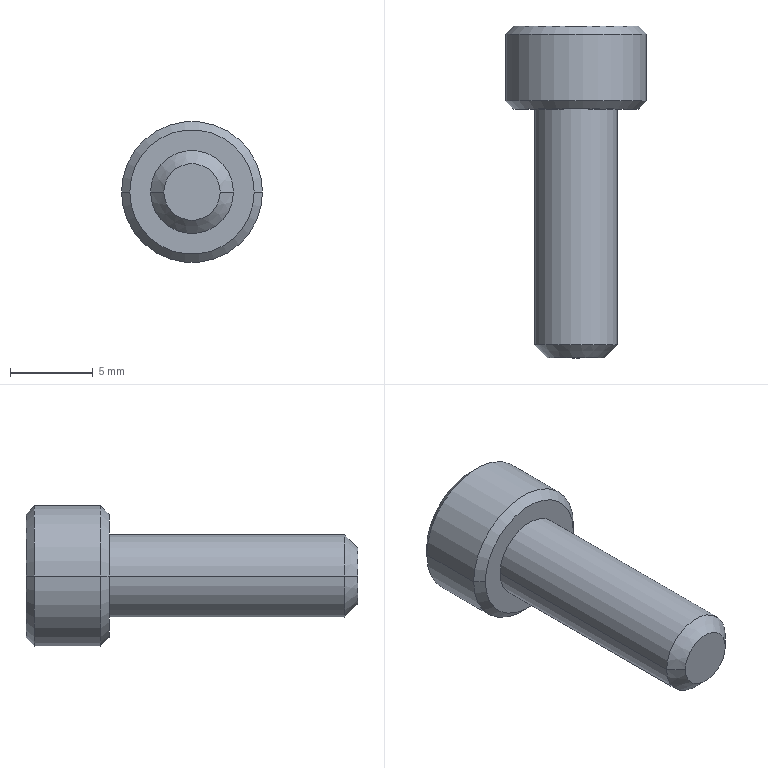Part | STEP file | BB62-M5-15L-1 | 1 solid | 27 faces | box 8.5 x 20 x 8.5 mm | volume 526.023 mm3 | plane 15 | cone 8 | cylinder 4 | commonest cylinder face diameters 5 x2 8.5 x2
STEP:
#1=CARTESIAN_POINT('',(0.,1.178,0.));
#2=VERTEX_POINT('',#1);
#3=CARTESIAN_POINT('',(2.29,2.5,0.));
#4=VERTEX_POINT('',#3);
#5=CARTESIAN_POINT('',(0.,1.178,0.));
#6=DIRECTION('',(0.866,0.5,0.));
#7=VECTOR('',#6,1000.);
#8=LINE('',#5,#7);
#9=EDGE_CURVE('',#2,#4,#8,.T.);
#10=ORIENTED_EDGE('',*,*,#9,.F.);
#11=CARTESIAN_POINT('',(-2.29,2.5,0.));
#12=VERTEX_POINT('',#11);
#13=CARTESIAN_POINT('',(0.,1.178,0.));
#14=DIRECTION('',(-0.866,0.5,0.));
#15=VECTOR('',#14,1000.);
#16=LINE('',#13,#15);
#17=EDGE_CURVE('',#2,#12,#16,.T.);
#18=ORIENTED_EDGE('',*,*,#17,.T.);
#19=CARTESIAN_POINT('',(-1.983,2.5,1.145));
#20=VERTEX_POINT('',#19);
#21=CARTESIAN_POINT('',(0.,2.5,0.));
#22=DIRECTION('',(0.,-1.,0.));
#23=DIRECTION('',(-1.,0.,0.));
#24=AXIS2_PLACEMENT_3D('',#21,#22,#23);
#25=CIRCLE('',#24,2.29);
#26=EDGE_CURVE('',#20,#12,#25,.T.);
#27=ORIENTED_EDGE('',*,*,#26,.F.);
#28=CARTESIAN_POINT('',(0.,2.5,2.29));
#29=VERTEX_POINT('',#28);
#30=CARTESIAN_POINT('',(0.,2.5,0.));
#31=DIRECTION('',(0.,-1.,0.));
#32=DIRECTION('',(-1.,0.,0.));
#33=AXIS2_PLACEMENT_3D('',#30,#31,#32);
#34=CIRCLE('',#33,2.29);
#35=EDGE_CURVE('',#29,#20,#34,.T.);
#36=ORIENTED_EDGE('',*,*,#35,.F.);
#37=CARTESIAN_POINT('',(1.983,2.5,1.145));
#38=VERTEX_POINT('',#37);
#39=CARTESIAN_POINT('',(0.,2.5,0.));
#40=DIRECTION('',(0.,-1.,0.));
#41=DIRECTION('',(-1.,0.,0.));
#42=AXIS2_PLACEMENT_3D('',#39,#40,#41);
#43=CIRCLE('',#42,2.29);
#44=EDGE_CURVE('',#38,#29,#43,.T.);
#45=ORIENTED_EDGE('',*,*,#44,.F.);
#46=CARTESIAN_POINT('',(0.,2.5,0.));
#47=DIRECTION('',(0.,-1.,0.));
#48=DIRECTION('',(-1.,0.,0.));
#49=AXIS2_PLACEMENT_3D('',#46,#47,#48);
#50=CIRCLE('',#49,2.29);
#51=EDGE_CURVE('',#4,#38,#50,.T.);
#52=ORIENTED_EDGE('',*,*,#51,.F.);
#53=EDGE_LOOP('',(#10,#18,#27,#36,#45,#52));
#54=FACE_OUTER_BOUND('',#53,.T.);
#55=CARTESIAN_POINT('',(0.,1001.178,0.));
#56=DIRECTION('',(0.,1.,0.));
#57=DIRECTION('',(1.,0.,0.));
#58=AXIS2_PLACEMENT_3D('',#55,#56,#57);
#59=CONICAL_SURFACE('',#58,1732.051,1.047);
#60=ADVANCED_FACE('',(#54),#59,.F.);
#61=CARTESIAN_POINT('',(1.7,-15.,0.));
#62=VERTEX_POINT('',#61);
#63=CARTESIAN_POINT('',(-1.7,-15.,0.));
#64=VERTEX_POINT('',#63);
#65=CARTESIAN_POINT('',(0.,-15.,0.));
#66=DIRECTION('',(0.,1.,0.));
#67=DIRECTION('',(1.,0.,0.));
#68=AXIS2_PLACEMENT_3D('',#65,#66,#67);
#69=CIRCLE('',#68,1.7);
#70=EDGE_CURVE('',#62,#64,#69,.T.);
#71=ORIENTED_EDGE('',*,*,#70,.T.);
#72=CARTESIAN_POINT('',(-2.5,-14.2,0.));
#73=VERTEX_POINT('',#72);
#74=CARTESIAN_POINT('',(-1.7,-15.,0.));
#75=DIRECTION('',(-0.7071,0.7071,0.));
#76=VECTOR('',#75,1000.);
#77=LINE('',#74,#76);
#78=EDGE_CURVE('',#64,#73,#77,.T.);
#79=ORIENTED_EDGE('',*,*,#78,.T.);
#80=CARTESIAN_POINT('',(2.5,-14.2,0.));
#81=VERTEX_POINT('',#80);
#82=CARTESIAN_POINT('',(0.,-14.2,0.));
#83=DIRECTION('',(0.,-1.,0.));
#84=DIRECTION('',(-1.,0.,0.));
#85=AXIS2_PLACEMENT_3D('',#82,#83,#84);
#86=CIRCLE('',#85,2.5);
#87=EDGE_CURVE('',#73,#81,#86,.T.);
#88=ORIENTED_EDGE('',*,*,#87,.T.);
#89=CARTESIAN_POINT('',(1.7,-15.,0.));
#90=DIRECTION('',(0.7071,0.7071,0.));
#91=VECTOR('',#90,1000.);
#92=LINE('',#89,#91);
#93=EDGE_CURVE('',#62,#81,#92,.T.);
#94=ORIENTED_EDGE('',*,*,#93,.F.);
#95=EDGE_LOOP('',(#71,#79,#88,#94));
#96=FACE_OUTER_BOUND('',#95,.T.);
#97=CARTESIAN_POINT('',(0.,-15.,0.));
#98=DIRECTION('',(0.,1.,0.));
#99=DIRECTION('',(1.,0.,0.));
#100=AXIS2_PLACEMENT_3D('',#97,#98,#99);
#101=CONICAL_SURFACE('',#100,1.7,0.7854);
#102=ADVANCED_FACE('',(#96),#101,.T.);
#103=ORIENTED_EDGE('',*,*,#87,.F.);
#104=CARTESIAN_POINT('',(-2.5,0.,0.));
#105=VERTEX_POINT('',#104);
#106=CARTESIAN_POINT('',(-2.5,-14.2,0.));
#107=DIRECTION('',(0.,1.,0.));
#108=VECTOR('',#107,1000.);
#109=LINE('',#106,#108);
#110=EDGE_CURVE('',#73,#105,#109,.T.);
#111=ORIENTED_EDGE('',*,*,#110,.T.);
#112=CARTESIAN_POINT('',(2.5,0.,0.));
#113=VERTEX_POINT('',#112);
#114=CARTESIAN_POINT('',(0.,0.,0.));
#115=DIRECTION('',(0.,-1.,0.));
#116=DIRECTION('',(-1.,0.,0.));
#117=AXIS2_PLACEMENT_3D('',#114,#115,#116);
#118=CIRCLE('',#117,2.5);
#119=EDGE_CURVE('',#105,#113,#118,.T.);
#120=ORIENTED_EDGE('',*,*,#119,.T.);
#121=CARTESIAN_POINT('',(2.5,-14.2,0.));
#122=DIRECTION('',(0.,1.,0.));
#123=VECTOR('',#122,1000.);
#124=LINE('',#121,#123);
#125=EDGE_CURVE('',#81,#113,#124,.T.);
#126=ORIENTED_EDGE('',*,*,#125,.F.);
#127=EDGE_LOOP('',(#103,#111,#120,#126));
#128=FACE_OUTER_BOUND('',#127,.T.);
#129=CARTESIAN_POINT('',(0.,-14.2,0.));
#130=DIRECTION('',(0.,1.,0.));
#131=DIRECTION('',(1.,0.,0.));
#132=AXIS2_PLACEMENT_3D('',#129,#130,#131);
#133=CYLINDRICAL_SURFACE('',#132,2.5);
#134=ADVANCED_FACE('',(#128),#133,.T.);
#135=CARTESIAN_POINT('',(-3.75,5.,0.));
#136=VERTEX_POINT('',#135);
#137=CARTESIAN_POINT('',(3.75,5.,0.));
#138=VERTEX_POINT('',#137);
#139=CARTESIAN_POINT('',(0.,5.,0.));
#140=DIRECTION('',(0.,-1.,0.));
#141=DIRECTION('',(-1.,0.,0.));
#142=AXIS2_PLACEMENT_3D('',#139,#140,#141);
#143=CIRCLE('',#142,3.75);
#144=EDGE_CURVE('',#136,#138,#143,.T.);
#145=ORIENTED_EDGE('',*,*,#144,.T.);
#146=CARTESIAN_POINT('',(4.25,4.5,0.));
#147=VERTEX_POINT('',#146);
#148=CARTESIAN_POINT('',(4.25,4.5,0.));
#149=DIRECTION('',(0.7071,-0.7071,0.));
#150=VECTOR('',#149,1000.);
#151=LINE('',#148,#150);
#152=EDGE_CURVE('',#138,#147,#151,.T.);
#153=ORIENTED_EDGE('',*,*,#152,.T.);
#154=CARTESIAN_POINT('',(-4.25,4.5,0.));
#155=VERTEX_POINT('',#154);
#156=CARTESIAN_POINT('',(0.,4.5,0.));
#157=DIRECTION('',(0.,-1.,0.));
#158=DIRECTION('',(-1.,0.,0.));
#159=AXIS2_PLACEMENT_3D('',#156,#157,#158);
#160=CIRCLE('',#159,4.25);
#161=EDGE_CURVE('',#155,#147,#160,.T.);
#162=ORIENTED_EDGE('',*,*,#161,.F.);
#163=CARTESIAN_POINT('',(-4.25,4.5,0.));
#164=DIRECTION('',(-0.7071,-0.7071,0.));
#165=VECTOR('',#164,1000.);
#166=LINE('',#163,#165);
#167=EDGE_CURVE('',#136,#155,#166,.T.);
#168=ORIENTED_EDGE('',*,*,#167,.F.);
#169=EDGE_LOOP('',(#145,#153,#162,#168));
#170=FACE_OUTER_BOUND('',#169,.T.);
#171=CARTESIAN_POINT('',(0.,4.5,0.));
#172=DIRECTION('',(0.,-1.,0.));
#173=DIRECTION('',(-1.,0.,0.));
#174=AXIS2_PLACEMENT_3D('',#171,#172,#173);
#175=CONICAL_SURFACE('',#174,4.25,0.7854);
#176=ADVANCED_FACE('',(#170),#175,.T.);
#177=ORIENTED_EDGE('',*,*,#161,.T.);
#178=CARTESIAN_POINT('',(4.25,0.5,0.));
#179=VERTEX_POINT('',#178);
#180=CARTESIAN_POINT('',(4.25,1.62,0.));
#181=DIRECTION('',(0.,-1.,0.));
#182=VECTOR('',#181,1000.);
#183=LINE('',#180,#182);
#184=EDGE_CURVE('',#147,#179,#183,.T.);
#185=ORIENTED_EDGE('',*,*,#184,.T.);
#186=CARTESIAN_POINT('',(-4.25,0.5,0.));
#187=VERTEX_POINT('',#186);
#188=CARTESIAN_POINT('',(0.,0.5,0.));
#189=DIRECTION('',(0.,-1.,0.));
#190=DIRECTION('',(-1.,0.,0.));
#191=AXIS2_PLACEMENT_3D('',#188,#189,#190);
#192=CIRCLE('',#191,4.25);
#193=EDGE_CURVE('',#187,#179,#192,.T.);
#194=ORIENTED_EDGE('',*,*,#193,.F.);
#195=CARTESIAN_POINT('',(-4.25,1.62,0.));
#196=DIRECTION('',(0.,-1.,0.));
#197=VECTOR('',#196,1000.);
#198=LINE('',#195,#197);
#199=EDGE_CURVE('',#155,#187,#198,.T.);
#200=ORIENTED_EDGE('',*,*,#199,.F.);
#201=EDGE_LOOP('',(#177,#185,#194,#200));
#202=FACE_OUTER_BOUND('',#201,.T.);
#203=CARTESIAN_POINT('',(0.,1.62,0.));
#204=DIRECTION('',(0.,-1.,0.));
#205=DIRECTION('',(-1.,0.,0.));
#206=AXIS2_PLACEMENT_3D('',#203,#204,#205);
#207=CYLINDRICAL_SURFACE('',#206,4.25);
#208=ADVANCED_FACE('',(#202),#207,.T.);
#209=CARTESIAN_POINT('',(-3.75,0.,0.));
#210=VERTEX_POINT('',#209);
#211=CARTESIAN_POINT('',(3.75,0.,0.));
#212=VERTEX_POINT('',#211);
#213=CARTESIAN_POINT('',(0.,0.,0.));
#214=DIRECTION('',(0.,-1.,0.));
#215=DIRECTION('',(-1.,0.,0.));
#216=AXIS2_PLACEMENT_3D('',#213,#214,#215);
#217=CIRCLE('',#216,3.75);
#218=EDGE_CURVE('',#210,#212,#217,.T.);
#219=ORIENTED_EDGE('',*,*,#218,.F.);
#220=CARTESIAN_POINT('',(-3.75,0.,0.));
#221=DIRECTION('',(-0.7071,0.7071,0.));
#222=VECTOR('',#221,1000.);
#223=LINE('',#220,#222);
#224=EDGE_CURVE('',#210,#187,#223,.T.);
#225=ORIENTED_EDGE('',*,*,#224,.T.);
#226=ORIENTED_EDGE('',*,*,#193,.T.);
#227=CARTESIAN_POINT('',(3.75,0.,0.));
#228=DIRECTION('',(0.7071,0.7071,0.));
#229=VECTOR('',#228,1000.);
#230=LINE('',#227,#229);
#231=EDGE_CURVE('',#212,#179,#230,.T.);
#232=ORIENTED_EDGE('',*,*,#231,.F.);
#233=EDGE_LOOP('',(#219,#225,#226,#232));
#234=FACE_OUTER_BOUND('',#233,.T.);
#235=CARTESIAN_POINT('',(0.,0.,0.));
#236=DIRECTION('',(0.,1.,0.));
#237=DIRECTION('',(1.,0.,0.));
#238=AXIS2_PLACEMENT_3D('',#235,#236,#237);
#239=CONICAL_SURFACE('',#238,3.75,0.7854);
#240=ADVANCED_FACE('',(#234),#239,.T.);
#241=ORIENTED_EDGE('',*,*,#144,.F.);
#242=CARTESIAN_POINT('',(0.,5.,0.));
#243=DIRECTION('',(0.,-1.,0.));
#244=DIRECTION('',(-1.,0.,0.));
#245=AXIS2_PLACEMENT_3D('',#242,#243,#244);
#246=CIRCLE('',#245,3.75);
#247=EDGE_CURVE('',#138,#136,#246,.T.);
#248=ORIENTED_EDGE('',*,*,#247,.F.);
#249=EDGE_LOOP('',(#241,#248));
#250=FACE_OUTER_BOUND('',#249,.T.);
#251=CARTESIAN_POINT('',(0.,5.,-2.29));
#252=VERTEX_POINT('',#251);
#253=CARTESIAN_POINT('',(-1.983,5.,-1.145));
#254=VERTEX_POINT('',#253);
#255=CARTESIAN_POINT('',(0.,5.,-2.29));
#256=DIRECTION('',(-0.866,0.,0.5));
#257=VECTOR('',#256,1000.);
#258=LINE('',#255,#257);
#259=EDGE_CURVE('',#252,#254,#258,.T.);
#260=ORIENTED_EDGE('',*,*,#259,.F.);
#261=CARTESIAN_POINT('',(1.983,5.,-1.145));
#262=VERTEX_POINT('',#261);
#263=CARTESIAN_POINT('',(1.983,5.,-1.145));
#264=DIRECTION('',(-0.866,0.,-0.5));
#265=VECTOR('',#264,1000.);
#266=LINE('',#263,#265);
#267=EDGE_CURVE('',#262,#252,#266,.T.);
#268=ORIENTED_EDGE('',*,*,#267,.F.);
#269=CARTESIAN_POINT('',(1.983,5.,1.145));
#270=VERTEX_POINT('',#269);
#271=CARTESIAN_POINT('',(1.983,5.,1.145));
#272=DIRECTION('',(0.,0.,-1.));
#273=VECTOR('',#272,1000.);
#274=LINE('',#271,#273);
#275=EDGE_CURVE('',#270,#262,#274,.T.);
#276=ORIENTED_EDGE('',*,*,#275,.F.);
#277=CARTESIAN_POINT('',(0.,5.,2.29));
#278=VERTEX_POINT('',#277);
#279=CARTESIAN_POINT('',(0.,5.,2.29));
#280=DIRECTION('',(0.866,0.,-0.5));
#281=VECTOR('',#280,1000.);
#282=LINE('',#279,#281);
#283=EDGE_CURVE('',#278,#270,#282,.T.);
#284=ORIENTED_EDGE('',*,*,#283,.F.);
#285=CARTESIAN_POINT('',(-1.983,5.,1.145));
#286=VERTEX_POINT('',#285);
#287=CARTESIAN_POINT('',(-1.983,5.,1.145));
#288=DIRECTION('',(0.866,0.,0.5));
#289=VECTOR('',#288,1000.);
#290=LINE('',#287,#289);
#291=EDGE_CURVE('',#286,#278,#290,.T.);
#292=ORIENTED_EDGE('',*,*,#291,.F.);
#293=CARTESIAN_POINT('',(-1.983,5.,-1.145));
#294=DIRECTION('',(0.,0.,1.));
#295=VECTOR('',#294,1000.);
#296=LINE('',#293,#295);
#297=EDGE_CURVE('',#254,#286,#296,.T.);
#298=ORIENTED_EDGE('',*,*,#297,.F.);
#299=EDGE_LOOP('',(#260,#268,#276,#284,#292,#298));
#300=FACE_BOUND('',#299,.T.);
#301=CARTESIAN_POINT('',(3.75,5.,0.));
#302=DIRECTION('',(0.,1.,0.));
#303=DIRECTION('',(1.,0.,0.));
#304=AXIS2_PLACEMENT_3D('',#301,#302,#303);
#305=PLANE('',#304);
#306=ADVANCED_FACE('',(#250,#300),#305,.T.);
#307=CARTESIAN_POINT('',(0.,0.,0.));
#308=DIRECTION('',(0.,-1.,0.));
#309=DIRECTION('',(-1.,0.,0.));
#310=AXIS2_PLACEMENT_3D('',#307,#308,#309);
#311=CIRCLE('',#310,2.5);
#312=EDGE_CURVE('',#113,#105,#311,.T.);
#313=ORIENTED_EDGE('',*,*,#312,.F.);
#314=ORIENTED_EDGE('',*,*,#119,.F.);
#315=EDGE_LOOP('',(#313,#314));
#316=FACE_BOUND('',#315,.T.);
#317=CARTESIAN_POINT('',(0.,0.,0.));
#318=DIRECTION('',(0.,-1.,0.));
#319=DIRECTION('',(-1.,0.,0.));
#320=AXIS2_PLACEMENT_3D('',#317,#318,#319);
#321=CIRCLE('',#320,3.75);
#322=EDGE_CURVE('',#212,#210,#321,.T.);
#323=ORIENTED_EDGE('',*,*,#322,.T.);
#324=ORIENTED_EDGE('',*,*,#218,.T.);
#325=EDGE_LOOP('',(#323,#324));
#326=FACE_OUTER_BOUND('',#325,.T.);
#327=CARTESIAN_POINT('',(0.,0.,0.));
#328=DIRECTION('',(0.,-1.,0.));
#329=DIRECTION('',(-1.,0.,0.));
#330=AXIS2_PLACEMENT_3D('',#327,#328,#329);
#331=PLANE('',#330);
#332=ADVANCED_FACE('',(#316,#326),#331,.T.);
#333=ORIENTED_EDGE('',*,*,#224,.F.);
#334=ORIENTED_EDGE('',*,*,#322,.F.);
#335=ORIENTED_EDGE('',*,*,#231,.T.);
#336=CARTESIAN_POINT('',(0.,0.5,0.));
#337=DIRECTION('',(0.,-1.,0.));
#338=DIRECTION('',(-1.,0.,0.));
#339=AXIS2_PLACEMENT_3D('',#336,#337,#338);
#340=CIRCLE('',#339,4.25);
#341=EDGE_CURVE('',#179,#187,#340,.T.);
#342=ORIENTED_EDGE('',*,*,#341,.T.);
#343=EDGE_LOOP('',(#333,#334,#335,#342));
#344=FACE_OUTER_BOUND('',#343,.T.);
#345=CARTESIAN_POINT('',(0.,0.,0.));
#346=DIRECTION('',(0.,1.,0.));
#347=DIRECTION('',(1.,0.,0.));
#348=AXIS2_PLACEMENT_3D('',#345,#346,#347);
#349=CONICAL_SURFACE('',#348,3.75,0.7854);
#350=ADVANCED_FACE('',(#344),#349,.T.);
#351=ORIENTED_EDGE('',*,*,#184,.F.);
#352=CARTESIAN_POINT('',(0.,4.5,0.));
#353=DIRECTION('',(0.,-1.,0.));
#354=DIRECTION('',(-1.,0.,0.));
#355=AXIS2_PLACEMENT_3D('',#352,#353,#354);
#356=CIRCLE('',#355,4.25);
#357=EDGE_CURVE('',#147,#155,#356,.T.);
#358=ORIENTED_EDGE('',*,*,#357,.T.);
#359=ORIENTED_EDGE('',*,*,#199,.T.);
#360=ORIENTED_EDGE('',*,*,#341,.F.);
#361=EDGE_LOOP('',(#351,#358,#359,#360));
#362=FACE_OUTER_BOUND('',#361,.T.);
#363=CARTESIAN_POINT('',(0.,1.62,0.));
#364=DIRECTION('',(0.,-1.,0.));
#365=DIRECTION('',(-1.,0.,0.));
#366=AXIS2_PLACEMENT_3D('',#363,#364,#365);
#367=CYLINDRICAL_SURFACE('',#366,4.25);
#368=ADVANCED_FACE('',(#362),#367,.T.);
#369=ORIENTED_EDGE('',*,*,#152,.F.);
#370=ORIENTED_EDGE('',*,*,#247,.T.);
#371=ORIENTED_EDGE('',*,*,#167,.T.);
#372=ORIENTED_EDGE('',*,*,#357,.F.);
#373=EDGE_LOOP('',(#369,#370,#371,#372));
#374=FACE_OUTER_BOUND('',#373,.T.);
#375=CARTESIAN_POINT('',(0.,4.5,0.));
#376=DIRECTION('',(0.,-1.,0.));
#377=DIRECTION('',(-1.,0.,0.));
#378=AXIS2_PLACEMENT_3D('',#375,#376,#377);
#379=CONICAL_SURFACE('',#378,4.25,0.7854);
#380=ADVANCED_FACE('',(#374),#379,.T.);
#381=ORIENTED_EDGE('',*,*,#110,.F.);
#382=CARTESIAN_POINT('',(0.,-14.2,0.));
#383=DIRECTION('',(0.,-1.,0.));
#384=DIRECTION('',(-1.,0.,0.));
#385=AXIS2_PLACEMENT_3D('',#382,#383,#384);
#386=CIRCLE('',#385,2.5);
#387=EDGE_CURVE('',#81,#73,#386,.T.);
#388=ORIENTED_EDGE('',*,*,#387,.F.);
#389=ORIENTED_EDGE('',*,*,#125,.T.);
#390=ORIENTED_EDGE('',*,*,#312,.T.);
#391=EDGE_LOOP('',(#381,#388,#389,#390));
#392=FACE_OUTER_BOUND('',#391,.T.);
#393=CARTESIAN_POINT('',(0.,-14.2,0.));
#394=DIRECTION('',(0.,1.,0.));
#395=DIRECTION('',(1.,0.,0.));
#396=AXIS2_PLACEMENT_3D('',#393,#394,#395);
#397=CYLINDRICAL_SURFACE('',#396,2.5);
#398=ADVANCED_FACE('',(#392),#397,.T.);
#399=ORIENTED_EDGE('',*,*,#70,.F.);
#400=CARTESIAN_POINT('',(0.,-15.,0.));
#401=DIRECTION('',(0.,1.,0.));
#402=DIRECTION('',(1.,0.,0.));
#403=AXIS2_PLACEMENT_3D('',#400,#401,#402);
#404=CIRCLE('',#403,1.7);
#405=EDGE_CURVE('',#64,#62,#404,.T.);
#406=ORIENTED_EDGE('',*,*,#405,.F.);
#407=EDGE_LOOP('',(#399,#406));
#408=FACE_OUTER_BOUND('',#407,.T.);
#409=CARTESIAN_POINT('',(0.,-15.,0.));
#410=DIRECTION('',(0.,-1.,0.));
#411=DIRECTION('',(-1.,0.,0.));
#412=AXIS2_PLACEMENT_3D('',#409,#410,#411);
#413=PLANE('',#412);
#414=ADVANCED_FACE('',(#408),#413,.T.);
#415=ORIENTED_EDGE('',*,*,#78,.F.);
#416=ORIENTED_EDGE('',*,*,#405,.T.);
#417=ORIENTED_EDGE('',*,*,#93,.T.);
#418=ORIENTED_EDGE('',*,*,#387,.T.);
#419=EDGE_LOOP('',(#415,#416,#417,#418));
#420=FACE_OUTER_BOUND('',#419,.T.);
#421=CARTESIAN_POINT('',(0.,-15.,0.));
#422=DIRECTION('',(0.,1.,0.));
#423=DIRECTION('',(1.,0.,0.));
#424=AXIS2_PLACEMENT_3D('',#421,#422,#423);
#425=CONICAL_SURFACE('',#424,1.7,0.7854);
#426=ADVANCED_FACE('',(#420),#425,.T.);
#427=CARTESIAN_POINT('',(1.983,2.5,-1.145));
#428=VERTEX_POINT('',#427);
#429=CARTESIAN_POINT('',(0.,2.5,-2.29));
#430=VERTEX_POINT('',#429);
#431=CARTESIAN_POINT('',(1.983,2.5,-1.145));
#432=DIRECTION('',(-0.866,0.,-0.5));
#433=VECTOR('',#432,1000.);
#434=LINE('',#431,#433);
#435=EDGE_CURVE('',#428,#430,#434,.T.);
#436=ORIENTED_EDGE('',*,*,#435,.F.);
#437=CARTESIAN_POINT('',(1.983,5.,-1.145));
#438=DIRECTION('',(0.,-1.,0.));
#439=VECTOR('',#438,1000.);
#440=LINE('',#437,#439);
#441=EDGE_CURVE('',#262,#428,#440,.T.);
#442=ORIENTED_EDGE('',*,*,#441,.F.);
#443=ORIENTED_EDGE('',*,*,#267,.T.);
#444=CARTESIAN_POINT('',(0.,5.,-2.29));
#445=DIRECTION('',(0.,-1.,0.));
#446=VECTOR('',#445,1000.);
#447=LINE('',#444,#446);
#448=EDGE_CURVE('',#252,#430,#447,.T.);
#449=ORIENTED_EDGE('',*,*,#448,.T.);
#450=EDGE_LOOP('',(#436,#442,#443,#449));
#451=FACE_OUTER_BOUND('',#450,.T.);
#452=CARTESIAN_POINT('',(1.983,5.,-1.145));
#453=DIRECTION('',(-0.5,0.,0.866));
#454=DIRECTION('',(0.866,0.,0.5));
#455=AXIS2_PLACEMENT_3D('',#452,#453,#454);
#456=PLANE('',#455);
#457=ADVANCED_FACE('',(#451),#456,.T.);
#458=CARTESIAN_POINT('',(-1.983,2.5,-1.145));
#459=VERTEX_POINT('',#458);
#460=CARTESIAN_POINT('',(0.,2.5,-2.29));
#461=DIRECTION('',(-0.866,0.,0.5));
#462=VECTOR('',#461,1000.);
#463=LINE('',#460,#462);
#464=EDGE_CURVE('',#430,#459,#463,.T.);
#465=ORIENTED_EDGE('',*,*,#464,.F.);
#466=ORIENTED_EDGE('',*,*,#448,.F.);
#467=ORIENTED_EDGE('',*,*,#259,.T.);
#468=CARTESIAN_POINT('',(-1.983,5.,-1.145));
#469=DIRECTION('',(0.,-1.,0.));
#470=VECTOR('',#469,1000.);
#471=LINE('',#468,#470);
#472=EDGE_CURVE('',#254,#459,#471,.T.);
#473=ORIENTED_EDGE('',*,*,#472,.T.);
#474=EDGE_LOOP('',(#465,#466,#467,#473));
#475=FACE_OUTER_BOUND('',#474,.T.);
#476=CARTESIAN_POINT('',(0.,5.,-2.29));
#477=DIRECTION('',(0.5,0.,0.866));
#478=DIRECTION('',(0.866,0.,-0.5));
#479=AXIS2_PLACEMENT_3D('',#476,#477,#478);
#480=PLANE('',#479);
#481=ADVANCED_FACE('',(#475),#480,.T.);
#482=CARTESIAN_POINT('',(-1.983,2.5,-1.145));
#483=DIRECTION('',(0.,0.,1.));
#484=VECTOR('',#483,1000.);
#485=LINE('',#482,#484);
#486=EDGE_CURVE('',#459,#20,#485,.T.);
#487=ORIENTED_EDGE('',*,*,#486,.F.);
#488=ORIENTED_EDGE('',*,*,#472,.F.);
#489=ORIENTED_EDGE('',*,*,#297,.T.);
#490=CARTESIAN_POINT('',(-1.983,5.,1.145));
#491=DIRECTION('',(0.,-1.,0.));
#492=VECTOR('',#491,1000.);
#493=LINE('',#490,#492);
#494=EDGE_CURVE('',#286,#20,#493,.T.);
#495=ORIENTED_EDGE('',*,*,#494,.T.);
#496=EDGE_LOOP('',(#487,#488,#489,#495));
#497=FACE_OUTER_BOUND('',#496,.T.);
#498=CARTESIAN_POINT('',(-1.983,5.,-1.145));
#499=DIRECTION('',(1.,0.,0.));
#500=DIRECTION('',(0.,0.,-1.));
#501=AXIS2_PLACEMENT_3D('',#498,#499,#500);
#502=PLANE('',#501);
#503=ADVANCED_FACE('',(#497),#502,.T.);
#504=CARTESIAN_POINT('',(-1.983,2.5,1.145));
#505=DIRECTION('',(0.866,0.,0.5));
#506=VECTOR('',#505,1000.);
#507=LINE('',#504,#506);
#508=EDGE_CURVE('',#20,#29,#507,.T.);
#509=ORIENTED_EDGE('',*,*,#508,.F.);
#510=ORIENTED_EDGE('',*,*,#494,.F.);
#511=ORIENTED_EDGE('',*,*,#291,.T.);
#512=CARTESIAN_POINT('',(0.,5.,2.29));
#513=DIRECTION('',(0.,-1.,0.));
#514=VECTOR('',#513,1000.);
#515=LINE('',#512,#514);
#516=EDGE_CURVE('',#278,#29,#515,.T.);
#517=ORIENTED_EDGE('',*,*,#516,.T.);
#518=EDGE_LOOP('',(#509,#510,#511,#517));
#519=FACE_OUTER_BOUND('',#518,.T.);
#520=CARTESIAN_POINT('',(-1.983,5.,1.145));
#521=DIRECTION('',(0.5,0.,-0.866));
#522=DIRECTION('',(-0.866,0.,-0.5));
#523=AXIS2_PLACEMENT_3D('',#520,#521,#522);
#524=PLANE('',#523);
#525=ADVANCED_FACE('',(#519),#524,.T.);
#526=CARTESIAN_POINT('',(0.,2.5,2.29));
#527=DIRECTION('',(0.866,0.,-0.5));
#528=VECTOR('',#527,1000.);
#529=LINE('',#526,#528);
#530=EDGE_CURVE('',#29,#38,#529,.T.);
#531=ORIENTED_EDGE('',*,*,#530,.F.);
#532=ORIENTED_EDGE('',*,*,#516,.F.);
#533=ORIENTED_EDGE('',*,*,#283,.T.);
#534=CARTESIAN_POINT('',(1.983,5.,1.145));
#535=DIRECTION('',(0.,-1.,0.));
#536=VECTOR('',#535,1000.);
#537=LINE('',#534,#536);
#538=EDGE_CURVE('',#270,#38,#537,.T.);
#539=ORIENTED_EDGE('',*,*,#538,.T.);
#540=EDGE_LOOP('',(#531,#532,#533,#539));
#541=FACE_OUTER_BOUND('',#540,.T.);
#542=CARTESIAN_POINT('',(0.,5.,2.29));
#543=DIRECTION('',(-0.5,0.,-0.866));
#544=DIRECTION('',(-0.866,0.,0.5));
#545=AXIS2_PLACEMENT_3D('',#542,#543,#544);
#546=PLANE('',#545);
#547=ADVANCED_FACE('',(#541),#546,.T.);
#548=CARTESIAN_POINT('',(1.983,2.5,1.145));
#549=DIRECTION('',(0.,0.,-1.));
#550=VECTOR('',#549,1000.);
#551=LINE('',#548,#550);
#552=EDGE_CURVE('',#38,#428,#551,.T.);
#553=ORIENTED_EDGE('',*,*,#552,.F.);
#554=ORIENTED_EDGE('',*,*,#538,.F.);
#555=ORIENTED_EDGE('',*,*,#275,.T.);
#556=ORIENTED_EDGE('',*,*,#441,.T.);
#557=EDGE_LOOP('',(#553,#554,#555,#556));
#558=FACE_OUTER_BOUND('',#557,.T.);
#559=CARTESIAN_POINT('',(1.983,5.,1.145));
#560=DIRECTION('',(-1.,0.,0.));
#561=DIRECTION('',(0.,0.,1.));
#562=AXIS2_PLACEMENT_3D('',#559,#560,#561);
#563=PLANE('',#562);
#564=ADVANCED_FACE('',(#558),#563,.T.);
#565=ORIENTED_EDGE('',*,*,#435,.T.);
#566=CARTESIAN_POINT('',(0.,2.5,0.));
#567=DIRECTION('',(0.,-1.,0.));
#568=DIRECTION('',(-1.,0.,0.));
#569=AXIS2_PLACEMENT_3D('',#566,#567,#568);
#570=CIRCLE('',#569,2.29);
#571=EDGE_CURVE('',#430,#428,#570,.T.);
#572=ORIENTED_EDGE('',*,*,#571,.T.);
#573=EDGE_LOOP('',(#565,#572));
#574=FACE_OUTER_BOUND('',#573,.T.);
#575=CARTESIAN_POINT('',(0.,2.5,0.));
#576=DIRECTION('',(0.,1.,0.));
#577=DIRECTION('',(1.,0.,0.));
#578=AXIS2_PLACEMENT_3D('',#575,#576,#577);
#579=PLANE('',#578);
#580=ADVANCED_FACE('',(#574),#579,.F.);
#581=ORIENTED_EDGE('',*,*,#552,.T.);
#582=CARTESIAN_POINT('',(0.,2.5,0.));
#583=DIRECTION('',(0.,-1.,0.));
#584=DIRECTION('',(-1.,0.,0.));
#585=AXIS2_PLACEMENT_3D('',#582,#583,#584);
#586=CIRCLE('',#585,2.29);
#587=EDGE_CURVE('',#428,#4,#586,.T.);
#588=ORIENTED_EDGE('',*,*,#587,.T.);
#589=ORIENTED_EDGE('',*,*,#51,.T.);
#590=EDGE_LOOP('',(#581,#588,#589));
#591=FACE_OUTER_BOUND('',#590,.T.);
#592=CARTESIAN_POINT('',(0.,2.5,0.));
#593=DIRECTION('',(0.,1.,0.));
#594=DIRECTION('',(1.,0.,0.));
#595=AXIS2_PLACEMENT_3D('',#592,#593,#594);
#596=PLANE('',#595);
#597=ADVANCED_FACE('',(#591),#596,.F.);
#598=ORIENTED_EDGE('',*,*,#530,.T.);
#599=ORIENTED_EDGE('',*,*,#44,.T.);
#600=EDGE_LOOP('',(#598,#599));
#601=FACE_OUTER_BOUND('',#600,.T.);
#602=CARTESIAN_POINT('',(0.,2.5,0.));
#603=DIRECTION('',(0.,1.,0.));
#604=DIRECTION('',(1.,0.,0.));
#605=AXIS2_PLACEMENT_3D('',#602,#603,#604);
#606=PLANE('',#605);
#607=ADVANCED_FACE('',(#601),#606,.F.);
#608=ORIENTED_EDGE('',*,*,#508,.T.);
#609=ORIENTED_EDGE('',*,*,#35,.T.);
#610=EDGE_LOOP('',(#608,#609));
#611=FACE_OUTER_BOUND('',#610,.T.);
#612=CARTESIAN_POINT('',(0.,2.5,0.));
#613=DIRECTION('',(0.,1.,0.));
#614=DIRECTION('',(1.,0.,0.));
#615=AXIS2_PLACEMENT_3D('',#612,#613,#614);
#616=PLANE('',#615);
#617=ADVANCED_FACE('',(#611),#616,.F.);
#618=ORIENTED_EDGE('',*,*,#486,.T.);
#619=ORIENTED_EDGE('',*,*,#26,.T.);
#620=CARTESIAN_POINT('',(0.,2.5,0.));
#621=DIRECTION('',(0.,-1.,0.));
#622=DIRECTION('',(-1.,0.,0.));
#623=AXIS2_PLACEMENT_3D('',#620,#621,#622);
#624=CIRCLE('',#623,2.29);
#625=EDGE_CURVE('',#12,#459,#624,.T.);
#626=ORIENTED_EDGE('',*,*,#625,.T.);
#627=EDGE_LOOP('',(#618,#619,#626));
#628=FACE_OUTER_BOUND('',#627,.T.);
#629=CARTESIAN_POINT('',(0.,2.5,0.));
#630=DIRECTION('',(0.,1.,0.));
#631=DIRECTION('',(1.,0.,0.));
#632=AXIS2_PLACEMENT_3D('',#629,#630,#631);
#633=PLANE('',#632);
#634=ADVANCED_FACE('',(#628),#633,.F.);
#635=ORIENTED_EDGE('',*,*,#464,.T.);
#636=CARTESIAN_POINT('',(0.,2.5,0.));
#637=DIRECTION('',(0.,-1.,0.));
#638=DIRECTION('',(-1.,0.,0.));
#639=AXIS2_PLACEMENT_3D('',#636,#637,#638);
#640=CIRCLE('',#639,2.29);
#641=EDGE_CURVE('',#459,#430,#640,.T.);
#642=ORIENTED_EDGE('',*,*,#641,.T.);
#643=EDGE_LOOP('',(#635,#642));
#644=FACE_OUTER_BOUND('',#643,.T.);
#645=CARTESIAN_POINT('',(0.,2.5,0.));
#646=DIRECTION('',(0.,1.,0.));
#647=DIRECTION('',(1.,0.,0.));
#648=AXIS2_PLACEMENT_3D('',#645,#646,#647);
#649=PLANE('',#648);
#650=ADVANCED_FACE('',(#644),#649,.F.);
#651=ORIENTED_EDGE('',*,*,#17,.F.);
#652=ORIENTED_EDGE('',*,*,#9,.T.);
#653=ORIENTED_EDGE('',*,*,#587,.F.);
#654=ORIENTED_EDGE('',*,*,#571,.F.);
#655=ORIENTED_EDGE('',*,*,#641,.F.);
#656=ORIENTED_EDGE('',*,*,#625,.F.);
#657=EDGE_LOOP('',(#651,#652,#653,#654,#655,#656));
#658=FACE_OUTER_BOUND('',#657,.T.);
#659=CARTESIAN_POINT('',(0.,1001.178,0.));
#660=DIRECTION('',(0.,1.,0.));
#661=DIRECTION('',(1.,0.,0.));
#662=AXIS2_PLACEMENT_3D('',#659,#660,#661);
#663=CONICAL_SURFACE('',#662,1732.051,1.047);
#664=ADVANCED_FACE('',(#658),#663,.F.);
#665=CLOSED_SHELL('',(#60,#102,#134,#176,#208,#240,#306,#332,#350,#368,#380,#398,#414,#426,#457,#481,#503,#525,#547,#564,#580,#597,#607,#617,#634,#650,#664));
#666=MANIFOLD_SOLID_BREP('',#665);
#667=CARTESIAN_POINT('',(0.,0.,0.));
#668=DIRECTION('',(0.,0.,1.));
#669=DIRECTION('',(1.,0.,0.));
#670=AXIS2_PLACEMENT_3D('',#667,#668,#669);
#671=(LENGTH_UNIT()NAMED_UNIT(*)SI_UNIT(.MILLI.,.METRE.));
#672=UNCERTAINTY_MEASURE_WITH_UNIT(LENGTH_MEASURE(0.00001),#671,'','');
#673=(NAMED_UNIT(*)PLANE_ANGLE_UNIT()SI_UNIT($,.RADIAN.));
#674=(NAMED_UNIT(*)SI_UNIT($,.STERADIAN.)SOLID_ANGLE_UNIT());
#675=(GEOMETRIC_REPRESENTATION_CONTEXT(3)GLOBAL_UNCERTAINTY_ASSIGNED_CONTEXT((#672))GLOBAL_UNIT_ASSIGNED_CONTEXT((#671,#673,#674))REPRESENTATION_CONTEXT('',''));
#676=ADVANCED_BREP_SHAPE_REPRESENTATION('',(#666,#670),#675);